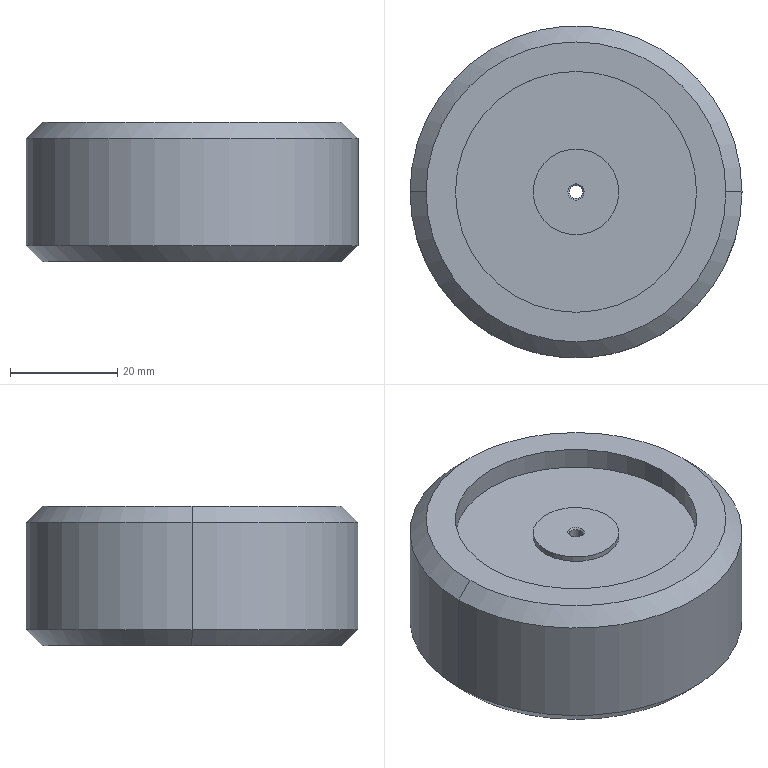Part | SolidWorks | features ICE 4, Chamfer 1, Extrusion 1, HoleWzd 1 | 1 solid | 28 faces | box 62 x 62 x 26 mm | volume 52713 mm3 | plane 12 | cylinder 10 | cone 6 | commonest cylinder face diameters 45 x4 2.5 x2 16 x2 62 x2
STEP:
#1=CARTESIAN_POINT('',(-28.,0.,0.));
#2=VERTEX_POINT('',#1);
#3=CARTESIAN_POINT('',(28.,0.,0.));
#4=VERTEX_POINT('',#3);
#5=CARTESIAN_POINT('',(0.,0.,0.));
#6=DIRECTION('',(0.,0.,-1.));
#7=DIRECTION('',(1.,0.,0.));
#8=AXIS2_PLACEMENT_3D('',#5,#6,#7);
#9=CIRCLE('',#8,28.);
#10=EDGE_CURVE('',#2,#4,#9,.T.);
#11=ORIENTED_EDGE('',*,*,#10,.F.);
#12=CARTESIAN_POINT('',(-31.,0.,3.));
#13=VERTEX_POINT('',#12);
#14=CARTESIAN_POINT('',(-31.,0.,3.));
#15=DIRECTION('',(-0.7071,0.,0.7071));
#16=VECTOR('',#15,1000.);
#17=LINE('',#14,#16);
#18=EDGE_CURVE('',#2,#13,#17,.T.);
#19=ORIENTED_EDGE('',*,*,#18,.T.);
#20=CARTESIAN_POINT('',(31.,0.,3.));
#21=VERTEX_POINT('',#20);
#22=CARTESIAN_POINT('',(0.,0.,3.));
#23=DIRECTION('',(0.,0.,1.));
#24=DIRECTION('',(1.,0.,0.));
#25=AXIS2_PLACEMENT_3D('',#22,#23,#24);
#26=CIRCLE('',#25,31.);
#27=EDGE_CURVE('',#21,#13,#26,.T.);
#28=ORIENTED_EDGE('',*,*,#27,.F.);
#29=CARTESIAN_POINT('',(31.,0.,3.));
#30=DIRECTION('',(0.7071,0.,0.7071));
#31=VECTOR('',#30,1000.);
#32=LINE('',#29,#31);
#33=EDGE_CURVE('',#4,#21,#32,.T.);
#34=ORIENTED_EDGE('',*,*,#33,.F.);
#35=EDGE_LOOP('',(#11,#19,#28,#34));
#36=FACE_OUTER_BOUND('',#35,.T.);
#37=CARTESIAN_POINT('',(0.,0.,3.));
#38=DIRECTION('',(0.,0.,1.));
#39=DIRECTION('',(1.,0.,0.));
#40=AXIS2_PLACEMENT_3D('',#37,#38,#39);
#41=CONICAL_SURFACE('',#40,31.,0.7854);
#42=ADVANCED_FACE('',(#36),#41,.T.);
#43=CARTESIAN_POINT('',(28.,0.,26.));
#44=VERTEX_POINT('',#43);
#45=CARTESIAN_POINT('',(-28.,0.,26.));
#46=VERTEX_POINT('',#45);
#47=CARTESIAN_POINT('',(0.,0.,26.));
#48=DIRECTION('',(0.,0.,1.));
#49=DIRECTION('',(1.,0.,0.));
#50=AXIS2_PLACEMENT_3D('',#47,#48,#49);
#51=CIRCLE('',#50,28.);
#52=EDGE_CURVE('',#44,#46,#51,.T.);
#53=ORIENTED_EDGE('',*,*,#52,.F.);
#54=CARTESIAN_POINT('',(31.,0.,23.));
#55=VERTEX_POINT('',#54);
#56=CARTESIAN_POINT('',(28.,0.,26.));
#57=DIRECTION('',(0.7071,0.,-0.7071));
#58=VECTOR('',#57,1000.);
#59=LINE('',#56,#58);
#60=EDGE_CURVE('',#44,#55,#59,.T.);
#61=ORIENTED_EDGE('',*,*,#60,.T.);
#62=CARTESIAN_POINT('',(-31.,0.,23.));
#63=VERTEX_POINT('',#62);
#64=CARTESIAN_POINT('',(0.,0.,23.));
#65=DIRECTION('',(0.,0.,-1.));
#66=DIRECTION('',(1.,0.,0.));
#67=AXIS2_PLACEMENT_3D('',#64,#65,#66);
#68=CIRCLE('',#67,31.);
#69=EDGE_CURVE('',#63,#55,#68,.T.);
#70=ORIENTED_EDGE('',*,*,#69,.F.);
#71=CARTESIAN_POINT('',(-28.,0.,26.));
#72=DIRECTION('',(-0.7071,0.,-0.7071));
#73=VECTOR('',#72,1000.);
#74=LINE('',#71,#73);
#75=EDGE_CURVE('',#46,#63,#74,.T.);
#76=ORIENTED_EDGE('',*,*,#75,.F.);
#77=EDGE_LOOP('',(#53,#61,#70,#76));
#78=FACE_OUTER_BOUND('',#77,.T.);
#79=CARTESIAN_POINT('',(0.,0.,26.));
#80=DIRECTION('',(0.,0.,-1.));
#81=DIRECTION('',(-1.,0.,0.));
#82=AXIS2_PLACEMENT_3D('',#79,#80,#81);
#83=CONICAL_SURFACE('',#82,28.,0.7854);
#84=ADVANCED_FACE('',(#78),#83,.T.);
#85=CARTESIAN_POINT('',(-1.25,0.,22.725));
#86=VERTEX_POINT('',#85);
#87=CARTESIAN_POINT('',(1.25,0.,22.725));
#88=VERTEX_POINT('',#87);
#89=CARTESIAN_POINT('',(0.,0.,22.725));
#90=DIRECTION('',(0.,0.,1.));
#91=DIRECTION('',(1.,0.,0.));
#92=AXIS2_PLACEMENT_3D('',#89,#90,#91);
#93=CIRCLE('',#92,1.25);
#94=EDGE_CURVE('',#86,#88,#93,.T.);
#95=ORIENTED_EDGE('',*,*,#94,.F.);
#96=CARTESIAN_POINT('',(-1.525,0.,23.));
#97=VERTEX_POINT('',#96);
#98=CARTESIAN_POINT('',(-1.525,0.,23.));
#99=DIRECTION('',(-0.7071,0.,0.7071));
#100=VECTOR('',#99,1000.);
#101=LINE('',#98,#100);
#102=EDGE_CURVE('',#86,#97,#101,.T.);
#103=ORIENTED_EDGE('',*,*,#102,.T.);
#104=CARTESIAN_POINT('',(1.525,0.,23.));
#105=VERTEX_POINT('',#104);
#106=CARTESIAN_POINT('',(0.,0.,23.));
#107=DIRECTION('',(0.,0.,1.));
#108=DIRECTION('',(1.,0.,0.));
#109=AXIS2_PLACEMENT_3D('',#106,#107,#108);
#110=CIRCLE('',#109,1.525);
#111=EDGE_CURVE('',#97,#105,#110,.T.);
#112=ORIENTED_EDGE('',*,*,#111,.T.);
#113=CARTESIAN_POINT('',(1.525,0.,23.));
#114=DIRECTION('',(0.7071,0.,0.7071));
#115=VECTOR('',#114,1000.);
#116=LINE('',#113,#115);
#117=EDGE_CURVE('',#88,#105,#116,.T.);
#118=ORIENTED_EDGE('',*,*,#117,.F.);
#119=EDGE_LOOP('',(#95,#103,#112,#118));
#120=FACE_OUTER_BOUND('',#119,.T.);
#121=CARTESIAN_POINT('',(0.,0.,23.));
#122=DIRECTION('',(0.,0.,1.));
#123=DIRECTION('',(1.,0.,0.));
#124=AXIS2_PLACEMENT_3D('',#121,#122,#123);
#125=CONICAL_SURFACE('',#124,1.525,0.7854);
#126=ADVANCED_FACE('',(#120),#125,.F.);
#127=CARTESIAN_POINT('',(1.25,0.,14.1));
#128=VERTEX_POINT('',#127);
#129=CARTESIAN_POINT('',(-1.25,0.,14.1));
#130=VERTEX_POINT('',#129);
#131=CARTESIAN_POINT('',(0.,0.,14.1));
#132=DIRECTION('',(0.,0.,-1.));
#133=DIRECTION('',(-1.,0.,0.));
#134=AXIS2_PLACEMENT_3D('',#131,#132,#133);
#135=CIRCLE('',#134,1.25);
#136=EDGE_CURVE('',#128,#130,#135,.T.);
#137=ORIENTED_EDGE('',*,*,#136,.T.);
#138=CARTESIAN_POINT('',(-1.25,0.,23.));
#139=DIRECTION('',(0.,0.,1.));
#140=VECTOR('',#139,1000.);
#141=LINE('',#138,#140);
#142=EDGE_CURVE('',#130,#86,#141,.T.);
#143=ORIENTED_EDGE('',*,*,#142,.T.);
#144=ORIENTED_EDGE('',*,*,#94,.T.);
#145=CARTESIAN_POINT('',(1.25,0.,23.));
#146=DIRECTION('',(0.,0.,1.));
#147=VECTOR('',#146,1000.);
#148=LINE('',#145,#147);
#149=EDGE_CURVE('',#128,#88,#148,.T.);
#150=ORIENTED_EDGE('',*,*,#149,.F.);
#151=EDGE_LOOP('',(#137,#143,#144,#150));
#152=FACE_OUTER_BOUND('',#151,.T.);
#153=CARTESIAN_POINT('',(0.,0.,23.));
#154=DIRECTION('',(0.,0.,1.));
#155=DIRECTION('',(1.,0.,0.));
#156=AXIS2_PLACEMENT_3D('',#153,#154,#155);
#157=CYLINDRICAL_SURFACE('',#156,1.25);
#158=ADVANCED_FACE('',(#152),#157,.F.);
#159=CARTESIAN_POINT('',(-22.5,0.,22.));
#160=VERTEX_POINT('',#159);
#161=CARTESIAN_POINT('',(22.5,0.,22.));
#162=VERTEX_POINT('',#161);
#163=CARTESIAN_POINT('',(0.,0.,22.));
#164=DIRECTION('',(0.,0.,1.));
#165=DIRECTION('',(1.,0.,0.));
#166=AXIS2_PLACEMENT_3D('',#163,#164,#165);
#167=CIRCLE('',#166,22.5);
#168=EDGE_CURVE('',#160,#162,#167,.T.);
#169=ORIENTED_EDGE('',*,*,#168,.F.);
#170=CARTESIAN_POINT('',(-22.5,0.,26.));
#171=VERTEX_POINT('',#170);
#172=CARTESIAN_POINT('',(-22.5,0.,22.));
#173=DIRECTION('',(0.,0.,1.));
#174=VECTOR('',#173,1000.);
#175=LINE('',#172,#174);
#176=EDGE_CURVE('',#160,#171,#175,.T.);
#177=ORIENTED_EDGE('',*,*,#176,.T.);
#178=CARTESIAN_POINT('',(22.5,0.,26.));
#179=VERTEX_POINT('',#178);
#180=CARTESIAN_POINT('',(0.,0.,26.));
#181=DIRECTION('',(0.,0.,1.));
#182=DIRECTION('',(1.,0.,0.));
#183=AXIS2_PLACEMENT_3D('',#180,#181,#182);
#184=CIRCLE('',#183,22.5);
#185=EDGE_CURVE('',#171,#179,#184,.T.);
#186=ORIENTED_EDGE('',*,*,#185,.T.);
#187=CARTESIAN_POINT('',(22.5,0.,22.));
#188=DIRECTION('',(0.,0.,1.));
#189=VECTOR('',#188,1000.);
#190=LINE('',#187,#189);
#191=EDGE_CURVE('',#162,#179,#190,.T.);
#192=ORIENTED_EDGE('',*,*,#191,.F.);
#193=EDGE_LOOP('',(#169,#177,#186,#192));
#194=FACE_OUTER_BOUND('',#193,.T.);
#195=CARTESIAN_POINT('',(0.,0.,22.));
#196=DIRECTION('',(0.,0.,1.));
#197=DIRECTION('',(1.,0.,0.));
#198=AXIS2_PLACEMENT_3D('',#195,#196,#197);
#199=CYLINDRICAL_SURFACE('',#198,22.5);
#200=ADVANCED_FACE('',(#194),#199,.F.);
#201=CARTESIAN_POINT('',(22.5,0.,11.));
#202=VERTEX_POINT('',#201);
#203=CARTESIAN_POINT('',(-22.5,0.,11.));
#204=VERTEX_POINT('',#203);
#205=CARTESIAN_POINT('',(0.,0.,11.));
#206=DIRECTION('',(0.,0.,-1.));
#207=DIRECTION('',(-1.,0.,0.));
#208=AXIS2_PLACEMENT_3D('',#205,#206,#207);
#209=CIRCLE('',#208,22.5);
#210=EDGE_CURVE('',#202,#204,#209,.T.);
#211=ORIENTED_EDGE('',*,*,#210,.F.);
#212=CARTESIAN_POINT('',(22.5,0.,0.));
#213=VERTEX_POINT('',#212);
#214=CARTESIAN_POINT('',(22.5,0.,11.));
#215=DIRECTION('',(0.,0.,-1.));
#216=VECTOR('',#215,1000.);
#217=LINE('',#214,#216);
#218=EDGE_CURVE('',#202,#213,#217,.T.);
#219=ORIENTED_EDGE('',*,*,#218,.T.);
#220=CARTESIAN_POINT('',(-22.5,0.,0.));
#221=VERTEX_POINT('',#220);
#222=CARTESIAN_POINT('',(0.,0.,0.));
#223=DIRECTION('',(0.,0.,-1.));
#224=DIRECTION('',(-1.,0.,0.));
#225=AXIS2_PLACEMENT_3D('',#222,#223,#224);
#226=CIRCLE('',#225,22.5);
#227=EDGE_CURVE('',#213,#221,#226,.T.);
#228=ORIENTED_EDGE('',*,*,#227,.T.);
#229=CARTESIAN_POINT('',(-22.5,0.,11.));
#230=DIRECTION('',(0.,0.,-1.));
#231=VECTOR('',#230,1000.);
#232=LINE('',#229,#231);
#233=EDGE_CURVE('',#204,#221,#232,.T.);
#234=ORIENTED_EDGE('',*,*,#233,.F.);
#235=EDGE_LOOP('',(#211,#219,#228,#234));
#236=FACE_OUTER_BOUND('',#235,.T.);
#237=CARTESIAN_POINT('',(0.,0.,11.));
#238=DIRECTION('',(0.,0.,-1.));
#239=DIRECTION('',(-1.,0.,0.));
#240=AXIS2_PLACEMENT_3D('',#237,#238,#239);
#241=CYLINDRICAL_SURFACE('',#240,22.5);
#242=ADVANCED_FACE('',(#236),#241,.F.);
#243=ORIENTED_EDGE('',*,*,#69,.T.);
#244=CARTESIAN_POINT('',(31.,0.,26.));
#245=DIRECTION('',(0.,0.,-1.));
#246=VECTOR('',#245,1000.);
#247=LINE('',#244,#246);
#248=EDGE_CURVE('',#55,#21,#247,.T.);
#249=ORIENTED_EDGE('',*,*,#248,.T.);
#250=ORIENTED_EDGE('',*,*,#27,.T.);
#251=CARTESIAN_POINT('',(-31.,0.,26.));
#252=DIRECTION('',(0.,0.,-1.));
#253=VECTOR('',#252,1000.);
#254=LINE('',#251,#253);
#255=EDGE_CURVE('',#63,#13,#254,.T.);
#256=ORIENTED_EDGE('',*,*,#255,.F.);
#257=EDGE_LOOP('',(#243,#249,#250,#256));
#258=FACE_OUTER_BOUND('',#257,.T.);
#259=CARTESIAN_POINT('',(0.,0.,26.));
#260=DIRECTION('',(0.,0.,-1.));
#261=DIRECTION('',(-1.,0.,0.));
#262=AXIS2_PLACEMENT_3D('',#259,#260,#261);
#263=CYLINDRICAL_SURFACE('',#262,31.);
#264=ADVANCED_FACE('',(#258),#263,.T.);
#265=CARTESIAN_POINT('',(8.,0.,22.));
#266=VERTEX_POINT('',#265);
#267=CARTESIAN_POINT('',(-8.,0.,22.));
#268=VERTEX_POINT('',#267);
#269=CARTESIAN_POINT('',(0.,0.,22.));
#270=DIRECTION('',(0.,0.,1.));
#271=DIRECTION('',(1.,0.,0.));
#272=AXIS2_PLACEMENT_3D('',#269,#270,#271);
#273=CIRCLE('',#272,8.);
#274=EDGE_CURVE('',#266,#268,#273,.T.);
#275=ORIENTED_EDGE('',*,*,#274,.T.);
#276=CARTESIAN_POINT('',(-8.,0.,23.));
#277=VERTEX_POINT('',#276);
#278=CARTESIAN_POINT('',(-8.,0.,22.));
#279=DIRECTION('',(0.,0.,1.));
#280=VECTOR('',#279,1000.);
#281=LINE('',#278,#280);
#282=EDGE_CURVE('',#268,#277,#281,.T.);
#283=ORIENTED_EDGE('',*,*,#282,.T.);
#284=CARTESIAN_POINT('',(8.,0.,23.));
#285=VERTEX_POINT('',#284);
#286=CARTESIAN_POINT('',(0.,0.,23.));
#287=DIRECTION('',(0.,0.,1.));
#288=DIRECTION('',(1.,0.,0.));
#289=AXIS2_PLACEMENT_3D('',#286,#287,#288);
#290=CIRCLE('',#289,8.);
#291=EDGE_CURVE('',#285,#277,#290,.T.);
#292=ORIENTED_EDGE('',*,*,#291,.F.);
#293=CARTESIAN_POINT('',(8.,0.,22.));
#294=DIRECTION('',(0.,0.,1.));
#295=VECTOR('',#294,1000.);
#296=LINE('',#293,#295);
#297=EDGE_CURVE('',#266,#285,#296,.T.);
#298=ORIENTED_EDGE('',*,*,#297,.F.);
#299=EDGE_LOOP('',(#275,#283,#292,#298));
#300=FACE_OUTER_BOUND('',#299,.T.);
#301=CARTESIAN_POINT('',(0.,0.,22.));
#302=DIRECTION('',(0.,0.,1.));
#303=DIRECTION('',(1.,0.,0.));
#304=AXIS2_PLACEMENT_3D('',#301,#302,#303);
#305=CYLINDRICAL_SURFACE('',#304,8.);
#306=ADVANCED_FACE('',(#300),#305,.T.);
#307=ORIENTED_EDGE('',*,*,#282,.F.);
#308=CARTESIAN_POINT('',(0.,0.,22.));
#309=DIRECTION('',(0.,0.,1.));
#310=DIRECTION('',(1.,0.,0.));
#311=AXIS2_PLACEMENT_3D('',#308,#309,#310);
#312=CIRCLE('',#311,8.);
#313=EDGE_CURVE('',#268,#266,#312,.T.);
#314=ORIENTED_EDGE('',*,*,#313,.T.);
#315=ORIENTED_EDGE('',*,*,#297,.T.);
#316=CARTESIAN_POINT('',(0.,0.,23.));
#317=DIRECTION('',(0.,0.,1.));
#318=DIRECTION('',(1.,0.,0.));
#319=AXIS2_PLACEMENT_3D('',#316,#317,#318);
#320=CIRCLE('',#319,8.);
#321=EDGE_CURVE('',#277,#285,#320,.T.);
#322=ORIENTED_EDGE('',*,*,#321,.F.);
#323=EDGE_LOOP('',(#307,#314,#315,#322));
#324=FACE_OUTER_BOUND('',#323,.T.);
#325=CARTESIAN_POINT('',(0.,0.,22.));
#326=DIRECTION('',(0.,0.,1.));
#327=DIRECTION('',(1.,0.,0.));
#328=AXIS2_PLACEMENT_3D('',#325,#326,#327);
#329=CYLINDRICAL_SURFACE('',#328,8.);
#330=ADVANCED_FACE('',(#324),#329,.T.);
#331=ORIENTED_EDGE('',*,*,#248,.F.);
#332=CARTESIAN_POINT('',(0.,0.,23.));
#333=DIRECTION('',(0.,0.,-1.));
#334=DIRECTION('',(1.,0.,0.));
#335=AXIS2_PLACEMENT_3D('',#332,#333,#334);
#336=CIRCLE('',#335,31.);
#337=EDGE_CURVE('',#55,#63,#336,.T.);
#338=ORIENTED_EDGE('',*,*,#337,.T.);
#339=ORIENTED_EDGE('',*,*,#255,.T.);
#340=CARTESIAN_POINT('',(0.,0.,3.));
#341=DIRECTION('',(0.,0.,1.));
#342=DIRECTION('',(1.,0.,0.));
#343=AXIS2_PLACEMENT_3D('',#340,#341,#342);
#344=CIRCLE('',#343,31.);
#345=EDGE_CURVE('',#13,#21,#344,.T.);
#346=ORIENTED_EDGE('',*,*,#345,.T.);
#347=EDGE_LOOP('',(#331,#338,#339,#346));
#348=FACE_OUTER_BOUND('',#347,.T.);
#349=CARTESIAN_POINT('',(0.,0.,26.));
#350=DIRECTION('',(0.,0.,-1.));
#351=DIRECTION('',(-1.,0.,0.));
#352=AXIS2_PLACEMENT_3D('',#349,#350,#351);
#353=CYLINDRICAL_SURFACE('',#352,31.);
#354=ADVANCED_FACE('',(#348),#353,.T.);
#355=CARTESIAN_POINT('',(0.,0.,26.));
#356=DIRECTION('',(0.,0.,1.));
#357=DIRECTION('',(1.,0.,0.));
#358=AXIS2_PLACEMENT_3D('',#355,#356,#357);
#359=CIRCLE('',#358,28.);
#360=EDGE_CURVE('',#46,#44,#359,.T.);
#361=ORIENTED_EDGE('',*,*,#360,.T.);
#362=ORIENTED_EDGE('',*,*,#52,.T.);
#363=EDGE_LOOP('',(#361,#362));
#364=FACE_OUTER_BOUND('',#363,.T.);
#365=CARTESIAN_POINT('',(0.,0.,26.));
#366=DIRECTION('',(0.,0.,1.));
#367=DIRECTION('',(1.,0.,0.));
#368=AXIS2_PLACEMENT_3D('',#365,#366,#367);
#369=CIRCLE('',#368,22.5);
#370=EDGE_CURVE('',#179,#171,#369,.T.);
#371=ORIENTED_EDGE('',*,*,#370,.F.);
#372=ORIENTED_EDGE('',*,*,#185,.F.);
#373=EDGE_LOOP('',(#371,#372));
#374=FACE_BOUND('',#373,.T.);
#375=CARTESIAN_POINT('',(0.,0.,26.));
#376=DIRECTION('',(0.,0.,1.));
#377=DIRECTION('',(1.,0.,0.));
#378=AXIS2_PLACEMENT_3D('',#375,#376,#377);
#379=PLANE('',#378);
#380=ADVANCED_FACE('',(#364,#374),#379,.T.);
#381=CARTESIAN_POINT('',(0.,0.,0.));
#382=DIRECTION('',(0.,0.,-1.));
#383=DIRECTION('',(1.,0.,0.));
#384=AXIS2_PLACEMENT_3D('',#381,#382,#383);
#385=CIRCLE('',#384,28.);
#386=EDGE_CURVE('',#4,#2,#385,.T.);
#387=ORIENTED_EDGE('',*,*,#386,.T.);
#388=ORIENTED_EDGE('',*,*,#10,.T.);
#389=EDGE_LOOP('',(#387,#388));
#390=FACE_OUTER_BOUND('',#389,.T.);
#391=CARTESIAN_POINT('',(0.,0.,0.));
#392=DIRECTION('',(0.,0.,-1.));
#393=DIRECTION('',(-1.,0.,0.));
#394=AXIS2_PLACEMENT_3D('',#391,#392,#393);
#395=CIRCLE('',#394,22.5);
#396=EDGE_CURVE('',#221,#213,#395,.T.);
#397=ORIENTED_EDGE('',*,*,#396,.F.);
#398=ORIENTED_EDGE('',*,*,#227,.F.);
#399=EDGE_LOOP('',(#397,#398));
#400=FACE_BOUND('',#399,.T.);
#401=CARTESIAN_POINT('',(0.,0.,0.));
#402=DIRECTION('',(0.,0.,1.));
#403=DIRECTION('',(1.,0.,0.));
#404=AXIS2_PLACEMENT_3D('',#401,#402,#403);
#405=PLANE('',#404);
#406=ADVANCED_FACE('',(#390,#400),#405,.F.);
#407=ORIENTED_EDGE('',*,*,#218,.F.);
#408=CARTESIAN_POINT('',(0.,0.,11.));
#409=DIRECTION('',(0.,0.,-1.));
#410=DIRECTION('',(-1.,0.,0.));
#411=AXIS2_PLACEMENT_3D('',#408,#409,#410);
#412=CIRCLE('',#411,22.5);
#413=EDGE_CURVE('',#204,#202,#412,.T.);
#414=ORIENTED_EDGE('',*,*,#413,.F.);
#415=ORIENTED_EDGE('',*,*,#233,.T.);
#416=ORIENTED_EDGE('',*,*,#396,.T.);
#417=EDGE_LOOP('',(#407,#414,#415,#416));
#418=FACE_OUTER_BOUND('',#417,.T.);
#419=CARTESIAN_POINT('',(0.,0.,11.));
#420=DIRECTION('',(0.,0.,-1.));
#421=DIRECTION('',(-1.,0.,0.));
#422=AXIS2_PLACEMENT_3D('',#419,#420,#421);
#423=CYLINDRICAL_SURFACE('',#422,22.5);
#424=ADVANCED_FACE('',(#418),#423,.F.);
#425=CARTESIAN_POINT('',(-6.,3.464,11.));
#426=VERTEX_POINT('',#425);
#427=CARTESIAN_POINT('',(0.,6.928,11.));
#428=VERTEX_POINT('',#427);
#429=CARTESIAN_POINT('',(-6.,3.464,11.));
#430=DIRECTION('',(0.866,0.5,0.));
#431=VECTOR('',#430,1000.);
#432=LINE('',#429,#431);
#433=EDGE_CURVE('',#426,#428,#432,.T.);
#434=ORIENTED_EDGE('',*,*,#433,.F.);
#435=CARTESIAN_POINT('',(-6.,-3.464,11.));
#436=VERTEX_POINT('',#435);
#437=CARTESIAN_POINT('',(-6.,-3.464,11.));
#438=DIRECTION('',(0.,1.,0.));
#439=VECTOR('',#438,1000.);
#440=LINE('',#437,#439);
#441=EDGE_CURVE('',#436,#426,#440,.T.);
#442=ORIENTED_EDGE('',*,*,#441,.F.);
#443=CARTESIAN_POINT('',(0.,-6.928,11.));
#444=VERTEX_POINT('',#443);
#445=CARTESIAN_POINT('',(0.,-6.928,11.));
#446=DIRECTION('',(-0.866,0.5,0.));
#447=VECTOR('',#446,1000.);
#448=LINE('',#445,#447);
#449=EDGE_CURVE('',#444,#436,#448,.T.);
#450=ORIENTED_EDGE('',*,*,#449,.F.);
#451=CARTESIAN_POINT('',(6.,-3.464,11.));
#452=VERTEX_POINT('',#451);
#453=CARTESIAN_POINT('',(6.,-3.464,11.));
#454=DIRECTION('',(-0.866,-0.5,0.));
#455=VECTOR('',#454,1000.);
#456=LINE('',#453,#455);
#457=EDGE_CURVE('',#452,#444,#456,.T.);
#458=ORIENTED_EDGE('',*,*,#457,.F.);
#459=CARTESIAN_POINT('',(6.,3.464,11.));
#460=VERTEX_POINT('',#459);
#461=CARTESIAN_POINT('',(6.,3.464,11.));
#462=DIRECTION('',(0.,-1.,0.));
#463=VECTOR('',#462,1000.);
#464=LINE('',#461,#463);
#465=EDGE_CURVE('',#460,#452,#464,.T.);
#466=ORIENTED_EDGE('',*,*,#465,.F.);
#467=CARTESIAN_POINT('',(0.,6.928,11.));
#468=DIRECTION('',(0.866,-0.5,0.));
#469=VECTOR('',#468,1000.);
#470=LINE('',#467,#469);
#471=EDGE_CURVE('',#428,#460,#470,.T.);
#472=ORIENTED_EDGE('',*,*,#471,.F.);
#473=EDGE_LOOP('',(#434,#442,#450,#458,#466,#472));
#474=FACE_BOUND('',#473,.T.);
#475=ORIENTED_EDGE('',*,*,#413,.T.);
#476=ORIENTED_EDGE('',*,*,#210,.T.);
#477=EDGE_LOOP('',(#475,#476));
#478=FACE_OUTER_BOUND('',#477,.T.);
#479=CARTESIAN_POINT('',(0.,0.,11.));
#480=DIRECTION('',(0.,0.,-1.));
#481=DIRECTION('',(-1.,0.,0.));
#482=AXIS2_PLACEMENT_3D('',#479,#480,#481);
#483=PLANE('',#482);
#484=ADVANCED_FACE('',(#474,#478),#483,.T.);
#485=ORIENTED_EDGE('',*,*,#433,.T.);
#486=CARTESIAN_POINT('',(0.,6.928,14.1));
#487=VERTEX_POINT('',#486);
#488=CARTESIAN_POINT('',(0.,6.928,14.1));
#489=DIRECTION('',(0.,0.,-1.));
#490=VECTOR('',#489,1000.);
#491=LINE('',#488,#490);
#492=EDGE_CURVE('',#487,#428,#491,.T.);
#493=ORIENTED_EDGE('',*,*,#492,.F.);
#494=CARTESIAN_POINT('',(-6.,3.464,14.1));
#495=VERTEX_POINT('',#494);
#496=CARTESIAN_POINT('',(-6.,3.464,14.1));
#497=DIRECTION('',(0.866,0.5,0.));
#498=VECTOR('',#497,1000.);
#499=LINE('',#496,#498);
#500=EDGE_CURVE('',#495,#487,#499,.T.);
#501=ORIENTED_EDGE('',*,*,#500,.F.);
#502=CARTESIAN_POINT('',(-6.,3.464,14.1));
#503=DIRECTION('',(0.,0.,-1.));
#504=VECTOR('',#503,1000.);
#505=LINE('',#502,#504);
#506=EDGE_CURVE('',#495,#426,#505,.T.);
#507=ORIENTED_EDGE('',*,*,#506,.T.);
#508=EDGE_LOOP('',(#485,#493,#501,#507));
#509=FACE_OUTER_BOUND('',#508,.T.);
#510=CARTESIAN_POINT('',(-6.,3.464,14.1));
#511=DIRECTION('',(-0.5,0.866,0.));
#512=DIRECTION('',(-0.866,-0.5,0.));
#513=AXIS2_PLACEMENT_3D('',#510,#511,#512);
#514=PLANE('',#513);
#515=ADVANCED_FACE('',(#509),#514,.F.);
#516=ORIENTED_EDGE('',*,*,#441,.T.);
#517=ORIENTED_EDGE('',*,*,#506,.F.);
#518=CARTESIAN_POINT('',(-6.,-3.464,14.1));
#519=VERTEX_POINT('',#518);
#520=CARTESIAN_POINT('',(-6.,-3.464,14.1));
#521=DIRECTION('',(0.,1.,0.));
#522=VECTOR('',#521,1000.);
#523=LINE('',#520,#522);
#524=EDGE_CURVE('',#519,#495,#523,.T.);
#525=ORIENTED_EDGE('',*,*,#524,.F.);
#526=CARTESIAN_POINT('',(-6.,-3.464,14.1));
#527=DIRECTION('',(0.,0.,-1.));
#528=VECTOR('',#527,1000.);
#529=LINE('',#526,#528);
#530=EDGE_CURVE('',#519,#436,#529,.T.);
#531=ORIENTED_EDGE('',*,*,#530,.T.);
#532=EDGE_LOOP('',(#516,#517,#525,#531));
#533=FACE_OUTER_BOUND('',#532,.T.);
#534=CARTESIAN_POINT('',(-6.,-3.464,14.1));
#535=DIRECTION('',(-1.,0.,0.));
#536=DIRECTION('',(0.,-1.,0.));
#537=AXIS2_PLACEMENT_3D('',#534,#535,#536);
#538=PLANE('',#537);
#539=ADVANCED_FACE('',(#533),#538,.F.);
#540=ORIENTED_EDGE('',*,*,#449,.T.);
#541=ORIENTED_EDGE('',*,*,#530,.F.);
#542=CARTESIAN_POINT('',(0.,-6.928,14.1));
#543=VERTEX_POINT('',#542);
#544=CARTESIAN_POINT('',(0.,-6.928,14.1));
#545=DIRECTION('',(-0.866,0.5,0.));
#546=VECTOR('',#545,1000.);
#547=LINE('',#544,#546);
#548=EDGE_CURVE('',#543,#519,#547,.T.);
#549=ORIENTED_EDGE('',*,*,#548,.F.);
#550=CARTESIAN_POINT('',(0.,-6.928,14.1));
#551=DIRECTION('',(0.,0.,-1.));
#552=VECTOR('',#551,1000.);
#553=LINE('',#550,#552);
#554=EDGE_CURVE('',#543,#444,#553,.T.);
#555=ORIENTED_EDGE('',*,*,#554,.T.);
#556=EDGE_LOOP('',(#540,#541,#549,#555));
#557=FACE_OUTER_BOUND('',#556,.T.);
#558=CARTESIAN_POINT('',(0.,-6.928,14.1));
#559=DIRECTION('',(-0.5,-0.866,0.));
#560=DIRECTION('',(0.866,-0.5,0.));
#561=AXIS2_PLACEMENT_3D('',#558,#559,#560);
#562=PLANE('',#561);
#563=ADVANCED_FACE('',(#557),#562,.F.);
#564=ORIENTED_EDGE('',*,*,#457,.T.);
#565=ORIENTED_EDGE('',*,*,#554,.F.);
#566=CARTESIAN_POINT('',(6.,-3.464,14.1));
#567=VERTEX_POINT('',#566);
#568=CARTESIAN_POINT('',(6.,-3.464,14.1));
#569=DIRECTION('',(-0.866,-0.5,0.));
#570=VECTOR('',#569,1000.);
#571=LINE('',#568,#570);
#572=EDGE_CURVE('',#567,#543,#571,.T.);
#573=ORIENTED_EDGE('',*,*,#572,.F.);
#574=CARTESIAN_POINT('',(6.,-3.464,14.1));
#575=DIRECTION('',(0.,0.,-1.));
#576=VECTOR('',#575,1000.);
#577=LINE('',#574,#576);
#578=EDGE_CURVE('',#567,#452,#577,.T.);
#579=ORIENTED_EDGE('',*,*,#578,.T.);
#580=EDGE_LOOP('',(#564,#565,#573,#579));
#581=FACE_OUTER_BOUND('',#580,.T.);
#582=CARTESIAN_POINT('',(6.,-3.464,14.1));
#583=DIRECTION('',(0.5,-0.866,0.));
#584=DIRECTION('',(0.866,0.5,0.));
#585=AXIS2_PLACEMENT_3D('',#582,#583,#584);
#586=PLANE('',#585);
#587=ADVANCED_FACE('',(#581),#586,.F.);
#588=ORIENTED_EDGE('',*,*,#465,.T.);
#589=ORIENTED_EDGE('',*,*,#578,.F.);
#590=CARTESIAN_POINT('',(6.,3.464,14.1));
#591=VERTEX_POINT('',#590);
#592=CARTESIAN_POINT('',(6.,3.464,14.1));
#593=DIRECTION('',(0.,-1.,0.));
#594=VECTOR('',#593,1000.);
#595=LINE('',#592,#594);
#596=EDGE_CURVE('',#591,#567,#595,.T.);
#597=ORIENTED_EDGE('',*,*,#596,.F.);
#598=CARTESIAN_POINT('',(6.,3.464,14.1));
#599=DIRECTION('',(0.,0.,-1.));
#600=VECTOR('',#599,1000.);
#601=LINE('',#598,#600);
#602=EDGE_CURVE('',#591,#460,#601,.T.);
#603=ORIENTED_EDGE('',*,*,#602,.T.);
#604=EDGE_LOOP('',(#588,#589,#597,#603));
#605=FACE_OUTER_BOUND('',#604,.T.);
#606=CARTESIAN_POINT('',(6.,3.464,14.1));
#607=DIRECTION('',(1.,0.,0.));
#608=DIRECTION('',(0.,1.,0.));
#609=AXIS2_PLACEMENT_3D('',#606,#607,#608);
#610=PLANE('',#609);
#611=ADVANCED_FACE('',(#605),#610,.F.);
#612=ORIENTED_EDGE('',*,*,#471,.T.);
#613=ORIENTED_EDGE('',*,*,#602,.F.);
#614=CARTESIAN_POINT('',(0.,6.928,14.1));
#615=DIRECTION('',(0.866,-0.5,0.));
#616=VECTOR('',#615,1000.);
#617=LINE('',#614,#616);
#618=EDGE_CURVE('',#487,#591,#617,.T.);
#619=ORIENTED_EDGE('',*,*,#618,.F.);
#620=ORIENTED_EDGE('',*,*,#492,.T.);
#621=EDGE_LOOP('',(#612,#613,#619,#620));
#622=FACE_OUTER_BOUND('',#621,.T.);
#623=CARTESIAN_POINT('',(0.,6.928,14.1));
#624=DIRECTION('',(0.5,0.866,0.));
#625=DIRECTION('',(-0.866,0.5,0.));
#626=AXIS2_PLACEMENT_3D('',#623,#624,#625);
#627=PLANE('',#626);
#628=ADVANCED_FACE('',(#622),#627,.F.);
#629=ORIENTED_EDGE('',*,*,#136,.F.);
#630=CARTESIAN_POINT('',(0.,0.,14.1));
#631=DIRECTION('',(0.,0.,-1.));
#632=DIRECTION('',(-1.,0.,0.));
#633=AXIS2_PLACEMENT_3D('',#630,#631,#632);
#634=CIRCLE('',#633,1.25);
#635=EDGE_CURVE('',#130,#128,#634,.T.);
#636=ORIENTED_EDGE('',*,*,#635,.F.);
#637=EDGE_LOOP('',(#629,#636));
#638=FACE_BOUND('',#637,.T.);
#639=ORIENTED_EDGE('',*,*,#500,.T.);
#640=ORIENTED_EDGE('',*,*,#618,.T.);
#641=ORIENTED_EDGE('',*,*,#596,.T.);
#642=ORIENTED_EDGE('',*,*,#572,.T.);
#643=ORIENTED_EDGE('',*,*,#548,.T.);
#644=ORIENTED_EDGE('',*,*,#524,.T.);
#645=EDGE_LOOP('',(#639,#640,#641,#642,#643,#644));
#646=FACE_OUTER_BOUND('',#645,.T.);
#647=CARTESIAN_POINT('',(0.,0.,14.1));
#648=DIRECTION('',(0.,0.,-1.));
#649=DIRECTION('',(-1.,0.,0.));
#650=AXIS2_PLACEMENT_3D('',#647,#648,#649);
#651=PLANE('',#650);
#652=ADVANCED_FACE('',(#638,#646),#651,.T.);
#653=ORIENTED_EDGE('',*,*,#176,.F.);
#654=CARTESIAN_POINT('',(0.,0.,22.));
#655=DIRECTION('',(0.,0.,1.));
#656=DIRECTION('',(1.,0.,0.));
#657=AXIS2_PLACEMENT_3D('',#654,#655,#656);
#658=CIRCLE('',#657,22.5);
#659=EDGE_CURVE('',#162,#160,#658,.T.);
#660=ORIENTED_EDGE('',*,*,#659,.F.);
#661=ORIENTED_EDGE('',*,*,#191,.T.);
#662=ORIENTED_EDGE('',*,*,#370,.T.);
#663=EDGE_LOOP('',(#653,#660,#661,#662));
#664=FACE_OUTER_BOUND('',#663,.T.);
#665=CARTESIAN_POINT('',(0.,0.,22.));
#666=DIRECTION('',(0.,0.,1.));
#667=DIRECTION('',(1.,0.,0.));
#668=AXIS2_PLACEMENT_3D('',#665,#666,#667);
#669=CYLINDRICAL_SURFACE('',#668,22.5);
#670=ADVANCED_FACE('',(#664),#669,.F.);
#671=ORIENTED_EDGE('',*,*,#274,.F.);
#672=ORIENTED_EDGE('',*,*,#313,.F.);
#673=EDGE_LOOP('',(#671,#672));
#674=FACE_BOUND('',#673,.T.);
#675=ORIENTED_EDGE('',*,*,#659,.T.);
#676=ORIENTED_EDGE('',*,*,#168,.T.);
#677=EDGE_LOOP('',(#675,#676));
#678=FACE_OUTER_BOUND('',#677,.T.);
#679=CARTESIAN_POINT('',(0.,0.,22.));
#680=DIRECTION('',(0.,0.,1.));
#681=DIRECTION('',(1.,0.,0.));
#682=AXIS2_PLACEMENT_3D('',#679,#680,#681);
#683=PLANE('',#682);
#684=ADVANCED_FACE('',(#674,#678),#683,.T.);
#685=CARTESIAN_POINT('',(0.,0.,23.));
#686=DIRECTION('',(0.,0.,1.));
#687=DIRECTION('',(1.,0.,0.));
#688=AXIS2_PLACEMENT_3D('',#685,#686,#687);
#689=CIRCLE('',#688,1.525);
#690=EDGE_CURVE('',#105,#97,#689,.T.);
#691=ORIENTED_EDGE('',*,*,#690,.F.);
#692=ORIENTED_EDGE('',*,*,#111,.F.);
#693=EDGE_LOOP('',(#691,#692));
#694=FACE_BOUND('',#693,.T.);
#695=ORIENTED_EDGE('',*,*,#291,.T.);
#696=ORIENTED_EDGE('',*,*,#321,.T.);
#697=EDGE_LOOP('',(#695,#696));
#698=FACE_OUTER_BOUND('',#697,.T.);
#699=CARTESIAN_POINT('',(0.,0.,23.));
#700=DIRECTION('',(0.,0.,1.));
#701=DIRECTION('',(1.,0.,0.));
#702=AXIS2_PLACEMENT_3D('',#699,#700,#701);
#703=PLANE('',#702);
#704=ADVANCED_FACE('',(#694,#698),#703,.T.);
#705=ORIENTED_EDGE('',*,*,#142,.F.);
#706=ORIENTED_EDGE('',*,*,#635,.T.);
#707=ORIENTED_EDGE('',*,*,#149,.T.);
#708=CARTESIAN_POINT('',(0.,0.,22.725));
#709=DIRECTION('',(0.,0.,1.));
#710=DIRECTION('',(1.,0.,0.));
#711=AXIS2_PLACEMENT_3D('',#708,#709,#710);
#712=CIRCLE('',#711,1.25);
#713=EDGE_CURVE('',#88,#86,#712,.T.);
#714=ORIENTED_EDGE('',*,*,#713,.T.);
#715=EDGE_LOOP('',(#705,#706,#707,#714));
#716=FACE_OUTER_BOUND('',#715,.T.);
#717=CARTESIAN_POINT('',(0.,0.,23.));
#718=DIRECTION('',(0.,0.,1.));
#719=DIRECTION('',(1.,0.,0.));
#720=AXIS2_PLACEMENT_3D('',#717,#718,#719);
#721=CYLINDRICAL_SURFACE('',#720,1.25);
#722=ADVANCED_FACE('',(#716),#721,.F.);
#723=ORIENTED_EDGE('',*,*,#102,.F.);
#724=ORIENTED_EDGE('',*,*,#713,.F.);
#725=ORIENTED_EDGE('',*,*,#117,.T.);
#726=ORIENTED_EDGE('',*,*,#690,.T.);
#727=EDGE_LOOP('',(#723,#724,#725,#726));
#728=FACE_OUTER_BOUND('',#727,.T.);
#729=CARTESIAN_POINT('',(0.,0.,23.));
#730=DIRECTION('',(0.,0.,1.));
#731=DIRECTION('',(1.,0.,0.));
#732=AXIS2_PLACEMENT_3D('',#729,#730,#731);
#733=CONICAL_SURFACE('',#732,1.525,0.7854);
#734=ADVANCED_FACE('',(#728),#733,.F.);
#735=ORIENTED_EDGE('',*,*,#60,.F.);
#736=ORIENTED_EDGE('',*,*,#360,.F.);
#737=ORIENTED_EDGE('',*,*,#75,.T.);
#738=ORIENTED_EDGE('',*,*,#337,.F.);
#739=EDGE_LOOP('',(#735,#736,#737,#738));
#740=FACE_OUTER_BOUND('',#739,.T.);
#741=CARTESIAN_POINT('',(0.,0.,26.));
#742=DIRECTION('',(0.,0.,-1.));
#743=DIRECTION('',(-1.,0.,0.));
#744=AXIS2_PLACEMENT_3D('',#741,#742,#743);
#745=CONICAL_SURFACE('',#744,28.,0.7854);
#746=ADVANCED_FACE('',(#740),#745,.T.);
#747=ORIENTED_EDGE('',*,*,#18,.F.);
#748=ORIENTED_EDGE('',*,*,#386,.F.);
#749=ORIENTED_EDGE('',*,*,#33,.T.);
#750=ORIENTED_EDGE('',*,*,#345,.F.);
#751=EDGE_LOOP('',(#747,#748,#749,#750));
#752=FACE_OUTER_BOUND('',#751,.T.);
#753=CARTESIAN_POINT('',(0.,0.,3.));
#754=DIRECTION('',(0.,0.,1.));
#755=DIRECTION('',(1.,0.,0.));
#756=AXIS2_PLACEMENT_3D('',#753,#754,#755);
#757=CONICAL_SURFACE('',#756,31.,0.7854);
#758=ADVANCED_FACE('',(#752),#757,.T.);
#759=CLOSED_SHELL('',(#42,#84,#126,#158,#200,#242,#264,#306,#330,#354,#380,#406,#424,#484,#515,#539,#563,#587,#611,#628,#652,#670,#684,#704,#722,#734,#746,#758));
#760=MANIFOLD_SOLID_BREP('',#759);
#761=CARTESIAN_POINT('',(0.,0.,0.));
#762=DIRECTION('',(0.,0.,1.));
#763=DIRECTION('',(1.,0.,0.));
#764=AXIS2_PLACEMENT_3D('',#761,#762,#763);
#765=(LENGTH_UNIT()NAMED_UNIT(*)SI_UNIT(.MILLI.,.METRE.));
#766=UNCERTAINTY_MEASURE_WITH_UNIT(LENGTH_MEASURE(0.00001),#765,'','');
#767=(NAMED_UNIT(*)PLANE_ANGLE_UNIT()SI_UNIT($,.RADIAN.));
#768=(NAMED_UNIT(*)SI_UNIT($,.STERADIAN.)SOLID_ANGLE_UNIT());
#769=(GEOMETRIC_REPRESENTATION_CONTEXT(3)GLOBAL_UNCERTAINTY_ASSIGNED_CONTEXT((#766))GLOBAL_UNIT_ASSIGNED_CONTEXT((#765,#767,#768))REPRESENTATION_CONTEXT('',''));
#770=ADVANCED_BREP_SHAPE_REPRESENTATION('',(#760,#764),#769);